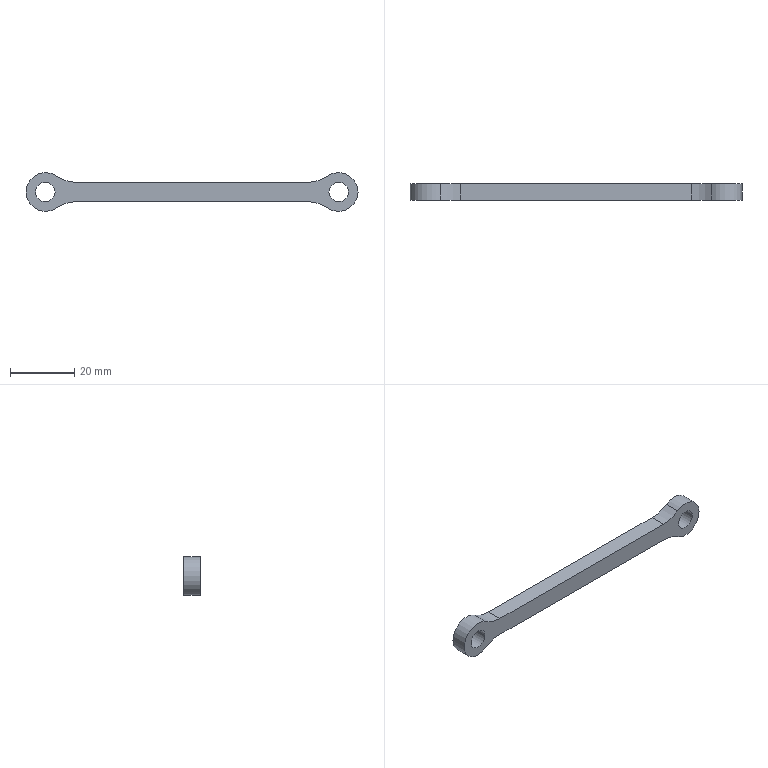Part | SolidWorks | features BaseBody 1 | 1 solid | 15 faces | box 103 x 5 x 12 mm | volume 3272 mm3 | cylinder 11 | plane 4 | commonest cylinder face diameters 6 x4 22 x4 12 x3
STEP:
#1=CARTESIAN_POINT('',(48.5,5.,0.));
#2=VERTEX_POINT('',#1);
#3=CARTESIAN_POINT('',(42.5,5.,0.));
#4=VERTEX_POINT('',#3);
#5=CARTESIAN_POINT('',(45.5,5.,0.));
#6=DIRECTION('',(0.,1.,0.));
#7=DIRECTION('',(1.,0.,0.));
#8=AXIS2_PLACEMENT_3D('',#5,#6,#7);
#9=CIRCLE('',#8,3.);
#10=EDGE_CURVE('',#2,#4,#9,.T.);
#11=ORIENTED_EDGE('',*,*,#10,.T.);
#12=CARTESIAN_POINT('',(42.5,0.,0.));
#13=VERTEX_POINT('',#12);
#14=CARTESIAN_POINT('',(42.5,5.,0.));
#15=DIRECTION('',(0.,-1.,0.));
#16=VECTOR('',#15,1000.);
#17=LINE('',#14,#16);
#18=EDGE_CURVE('',#4,#13,#17,.T.);
#19=ORIENTED_EDGE('',*,*,#18,.T.);
#20=CARTESIAN_POINT('',(48.5,0.,0.));
#21=VERTEX_POINT('',#20);
#22=CARTESIAN_POINT('',(45.5,0.,0.));
#23=DIRECTION('',(0.,-1.,0.));
#24=DIRECTION('',(1.,0.,0.));
#25=AXIS2_PLACEMENT_3D('',#22,#23,#24);
#26=CIRCLE('',#25,3.);
#27=EDGE_CURVE('',#13,#21,#26,.T.);
#28=ORIENTED_EDGE('',*,*,#27,.T.);
#29=CARTESIAN_POINT('',(48.5,5.,0.));
#30=DIRECTION('',(0.,-1.,0.));
#31=VECTOR('',#30,1000.);
#32=LINE('',#29,#31);
#33=EDGE_CURVE('',#2,#21,#32,.T.);
#34=ORIENTED_EDGE('',*,*,#33,.F.);
#35=EDGE_LOOP('',(#11,#19,#28,#34));
#36=FACE_OUTER_BOUND('',#35,.T.);
#37=CARTESIAN_POINT('',(45.5,5.,0.));
#38=DIRECTION('',(0.,-1.,0.));
#39=DIRECTION('',(1.,0.,0.));
#40=AXIS2_PLACEMENT_3D('',#37,#38,#39);
#41=CYLINDRICAL_SURFACE('',#40,3.);
#42=ADVANCED_FACE('',(#36),#41,.F.);
#43=CARTESIAN_POINT('',(-48.5,5.,0.));
#44=VERTEX_POINT('',#43);
#45=CARTESIAN_POINT('',(-42.5,5.,0.));
#46=VERTEX_POINT('',#45);
#47=CARTESIAN_POINT('',(-45.5,5.,0.));
#48=DIRECTION('',(0.,-1.,0.));
#49=DIRECTION('',(1.,0.,0.));
#50=AXIS2_PLACEMENT_3D('',#47,#48,#49);
#51=CIRCLE('',#50,3.);
#52=EDGE_CURVE('',#44,#46,#51,.T.);
#53=ORIENTED_EDGE('',*,*,#52,.F.);
#54=CARTESIAN_POINT('',(-48.5,0.,0.));
#55=VERTEX_POINT('',#54);
#56=CARTESIAN_POINT('',(-48.5,5.,0.));
#57=DIRECTION('',(0.,-1.,0.));
#58=VECTOR('',#57,1000.);
#59=LINE('',#56,#58);
#60=EDGE_CURVE('',#44,#55,#59,.T.);
#61=ORIENTED_EDGE('',*,*,#60,.T.);
#62=CARTESIAN_POINT('',(-42.5,0.,0.));
#63=VERTEX_POINT('',#62);
#64=CARTESIAN_POINT('',(-45.5,0.,0.));
#65=DIRECTION('',(0.,-1.,0.));
#66=DIRECTION('',(1.,0.,0.));
#67=AXIS2_PLACEMENT_3D('',#64,#65,#66);
#68=CIRCLE('',#67,3.);
#69=EDGE_CURVE('',#55,#63,#68,.T.);
#70=ORIENTED_EDGE('',*,*,#69,.T.);
#71=CARTESIAN_POINT('',(-42.5,5.,0.));
#72=DIRECTION('',(0.,-1.,0.));
#73=VECTOR('',#72,1000.);
#74=LINE('',#71,#73);
#75=EDGE_CURVE('',#46,#63,#74,.T.);
#76=ORIENTED_EDGE('',*,*,#75,.F.);
#77=EDGE_LOOP('',(#53,#61,#70,#76));
#78=FACE_OUTER_BOUND('',#77,.T.);
#79=CARTESIAN_POINT('',(-45.5,5.,0.));
#80=DIRECTION('',(0.,-1.,0.));
#81=DIRECTION('',(1.,0.,0.));
#82=AXIS2_PLACEMENT_3D('',#79,#80,#81);
#83=CYLINDRICAL_SURFACE('',#82,3.);
#84=ADVANCED_FACE('',(#78),#83,.F.);
#85=CARTESIAN_POINT('',(51.5,5.,0.));
#86=VERTEX_POINT('',#85);
#87=CARTESIAN_POINT('',(42.096,5.,-4.941));
#88=VERTEX_POINT('',#87);
#89=CARTESIAN_POINT('',(45.5,5.,0.));
#90=DIRECTION('',(0.,1.,0.));
#91=DIRECTION('',(1.,0.,0.));
#92=AXIS2_PLACEMENT_3D('',#89,#90,#91);
#93=CIRCLE('',#92,6.);
#94=EDGE_CURVE('',#86,#88,#93,.T.);
#95=ORIENTED_EDGE('',*,*,#94,.F.);
#96=CARTESIAN_POINT('',(51.5,0.,0.));
#97=VERTEX_POINT('',#96);
#98=CARTESIAN_POINT('',(51.5,5.,0.));
#99=DIRECTION('',(0.,-1.,0.));
#100=VECTOR('',#99,1000.);
#101=LINE('',#98,#100);
#102=EDGE_CURVE('',#86,#97,#101,.T.);
#103=ORIENTED_EDGE('',*,*,#102,.T.);
#104=CARTESIAN_POINT('',(42.096,0.,-4.941));
#105=VERTEX_POINT('',#104);
#106=CARTESIAN_POINT('',(45.5,0.,0.));
#107=DIRECTION('',(0.,1.,0.));
#108=DIRECTION('',(1.,0.,0.));
#109=AXIS2_PLACEMENT_3D('',#106,#107,#108);
#110=CIRCLE('',#109,6.);
#111=EDGE_CURVE('',#97,#105,#110,.T.);
#112=ORIENTED_EDGE('',*,*,#111,.T.);
#113=CARTESIAN_POINT('',(42.096,2.5,-4.941));
#114=DIRECTION('',(0.,-1.,0.));
#115=VECTOR('',#114,1000.);
#116=LINE('',#113,#115);
#117=EDGE_CURVE('',#88,#105,#116,.T.);
#118=ORIENTED_EDGE('',*,*,#117,.F.);
#119=EDGE_LOOP('',(#95,#103,#112,#118));
#120=FACE_OUTER_BOUND('',#119,.T.);
#121=CARTESIAN_POINT('',(45.5,5.,0.));
#122=DIRECTION('',(0.,-1.,0.));
#123=DIRECTION('',(1.,0.,0.));
#124=AXIS2_PLACEMENT_3D('',#121,#122,#123);
#125=CYLINDRICAL_SURFACE('',#124,6.);
#126=ADVANCED_FACE('',(#120),#125,.T.);
#127=ORIENTED_EDGE('',*,*,#18,.F.);
#128=CARTESIAN_POINT('',(45.5,5.,0.));
#129=DIRECTION('',(0.,1.,0.));
#130=DIRECTION('',(1.,0.,0.));
#131=AXIS2_PLACEMENT_3D('',#128,#129,#130);
#132=CIRCLE('',#131,3.);
#133=EDGE_CURVE('',#4,#2,#132,.T.);
#134=ORIENTED_EDGE('',*,*,#133,.T.);
#135=ORIENTED_EDGE('',*,*,#33,.T.);
#136=CARTESIAN_POINT('',(45.5,0.,0.));
#137=DIRECTION('',(0.,-1.,0.));
#138=DIRECTION('',(1.,0.,0.));
#139=AXIS2_PLACEMENT_3D('',#136,#137,#138);
#140=CIRCLE('',#139,3.);
#141=EDGE_CURVE('',#21,#13,#140,.T.);
#142=ORIENTED_EDGE('',*,*,#141,.T.);
#143=EDGE_LOOP('',(#127,#134,#135,#142));
#144=FACE_OUTER_BOUND('',#143,.T.);
#145=CARTESIAN_POINT('',(45.5,5.,0.));
#146=DIRECTION('',(0.,-1.,0.));
#147=DIRECTION('',(1.,0.,0.));
#148=AXIS2_PLACEMENT_3D('',#145,#146,#147);
#149=CYLINDRICAL_SURFACE('',#148,3.);
#150=ADVANCED_FACE('',(#144),#149,.F.);
#151=ORIENTED_EDGE('',*,*,#141,.F.);
#152=ORIENTED_EDGE('',*,*,#27,.F.);
#153=EDGE_LOOP('',(#151,#152));
#154=FACE_BOUND('',#153,.T.);
#155=CARTESIAN_POINT('',(-45.5,0.,0.));
#156=DIRECTION('',(0.,-1.,0.));
#157=DIRECTION('',(1.,0.,0.));
#158=AXIS2_PLACEMENT_3D('',#155,#156,#157);
#159=CIRCLE('',#158,3.);
#160=EDGE_CURVE('',#63,#55,#159,.T.);
#161=ORIENTED_EDGE('',*,*,#160,.F.);
#162=ORIENTED_EDGE('',*,*,#69,.F.);
#163=EDGE_LOOP('',(#161,#162));
#164=FACE_BOUND('',#163,.T.);
#165=CARTESIAN_POINT('',(42.096,0.,4.941));
#166=VERTEX_POINT('',#165);
#167=CARTESIAN_POINT('',(45.5,0.,0.));
#168=DIRECTION('',(0.,1.,0.));
#169=DIRECTION('',(1.,0.,0.));
#170=AXIS2_PLACEMENT_3D('',#167,#168,#169);
#171=CIRCLE('',#170,6.);
#172=EDGE_CURVE('',#166,#97,#171,.T.);
#173=ORIENTED_EDGE('',*,*,#172,.F.);
#174=CARTESIAN_POINT('',(35.856,0.,3.));
#175=VERTEX_POINT('',#174);
#176=CARTESIAN_POINT('',(35.856,0.,14.));
#177=DIRECTION('',(0.,-1.,0.));
#178=DIRECTION('',(1.,0.,0.));
#179=AXIS2_PLACEMENT_3D('',#176,#177,#178);
#180=CIRCLE('',#179,11.);
#181=EDGE_CURVE('',#175,#166,#180,.T.);
#182=ORIENTED_EDGE('',*,*,#181,.F.);
#183=CARTESIAN_POINT('',(-35.856,0.,3.));
#184=VERTEX_POINT('',#183);
#185=CARTESIAN_POINT('',(0.,0.,3.));
#186=DIRECTION('',(1.,0.,0.));
#187=VECTOR('',#186,1000.);
#188=LINE('',#185,#187);
#189=EDGE_CURVE('',#184,#175,#188,.T.);
#190=ORIENTED_EDGE('',*,*,#189,.F.);
#191=CARTESIAN_POINT('',(-42.096,0.,4.941));
#192=VERTEX_POINT('',#191);
#193=CARTESIAN_POINT('',(-35.856,0.,14.));
#194=DIRECTION('',(0.,-1.,0.));
#195=DIRECTION('',(1.,0.,0.));
#196=AXIS2_PLACEMENT_3D('',#193,#194,#195);
#197=CIRCLE('',#196,11.);
#198=EDGE_CURVE('',#192,#184,#197,.T.);
#199=ORIENTED_EDGE('',*,*,#198,.F.);
#200=CARTESIAN_POINT('',(-42.096,0.,-4.941));
#201=VERTEX_POINT('',#200);
#202=CARTESIAN_POINT('',(-45.5,0.,0.));
#203=DIRECTION('',(0.,1.,0.));
#204=DIRECTION('',(1.,0.,0.));
#205=AXIS2_PLACEMENT_3D('',#202,#203,#204);
#206=CIRCLE('',#205,6.);
#207=EDGE_CURVE('',#201,#192,#206,.T.);
#208=ORIENTED_EDGE('',*,*,#207,.F.);
#209=CARTESIAN_POINT('',(-35.856,0.,-3.));
#210=VERTEX_POINT('',#209);
#211=CARTESIAN_POINT('',(-35.856,0.,-14.));
#212=DIRECTION('',(0.,-1.,0.));
#213=DIRECTION('',(1.,0.,0.));
#214=AXIS2_PLACEMENT_3D('',#211,#212,#213);
#215=CIRCLE('',#214,11.);
#216=EDGE_CURVE('',#210,#201,#215,.T.);
#217=ORIENTED_EDGE('',*,*,#216,.F.);
#218=CARTESIAN_POINT('',(35.856,0.,-3.));
#219=VERTEX_POINT('',#218);
#220=CARTESIAN_POINT('',(0.,0.,-3.));
#221=DIRECTION('',(-1.,0.,0.));
#222=VECTOR('',#221,1000.);
#223=LINE('',#220,#222);
#224=EDGE_CURVE('',#219,#210,#223,.T.);
#225=ORIENTED_EDGE('',*,*,#224,.F.);
#226=CARTESIAN_POINT('',(35.856,0.,-14.));
#227=DIRECTION('',(0.,-1.,0.));
#228=DIRECTION('',(1.,0.,0.));
#229=AXIS2_PLACEMENT_3D('',#226,#227,#228);
#230=CIRCLE('',#229,11.);
#231=EDGE_CURVE('',#105,#219,#230,.T.);
#232=ORIENTED_EDGE('',*,*,#231,.F.);
#233=ORIENTED_EDGE('',*,*,#111,.F.);
#234=EDGE_LOOP('',(#173,#182,#190,#199,#208,#217,#225,#232,#233));
#235=FACE_OUTER_BOUND('',#234,.T.);
#236=CARTESIAN_POINT('',(-52.118,0.,-6.072));
#237=DIRECTION('',(0.,1.,0.));
#238=DIRECTION('',(0.,0.,1.));
#239=AXIS2_PLACEMENT_3D('',#236,#237,#238);
#240=PLANE('',#239);
#241=ADVANCED_FACE('',(#154,#164,#235),#240,.F.);
#242=ORIENTED_EDGE('',*,*,#10,.F.);
#243=ORIENTED_EDGE('',*,*,#133,.F.);
#244=EDGE_LOOP('',(#242,#243));
#245=FACE_BOUND('',#244,.T.);
#246=CARTESIAN_POINT('',(-45.5,5.,0.));
#247=DIRECTION('',(0.,-1.,0.));
#248=DIRECTION('',(1.,0.,0.));
#249=AXIS2_PLACEMENT_3D('',#246,#247,#248);
#250=CIRCLE('',#249,3.);
#251=EDGE_CURVE('',#46,#44,#250,.T.);
#252=ORIENTED_EDGE('',*,*,#251,.T.);
#253=ORIENTED_EDGE('',*,*,#52,.T.);
#254=EDGE_LOOP('',(#252,#253));
#255=FACE_BOUND('',#254,.T.);
#256=CARTESIAN_POINT('',(35.856,5.,3.));
#257=VERTEX_POINT('',#256);
#258=CARTESIAN_POINT('',(42.096,5.,4.941));
#259=VERTEX_POINT('',#258);
#260=CARTESIAN_POINT('',(35.856,5.,14.));
#261=DIRECTION('',(0.,-1.,0.));
#262=DIRECTION('',(1.,0.,0.));
#263=AXIS2_PLACEMENT_3D('',#260,#261,#262);
#264=CIRCLE('',#263,11.);
#265=EDGE_CURVE('',#257,#259,#264,.T.);
#266=ORIENTED_EDGE('',*,*,#265,.T.);
#267=CARTESIAN_POINT('',(45.5,5.,0.));
#268=DIRECTION('',(0.,1.,0.));
#269=DIRECTION('',(1.,0.,0.));
#270=AXIS2_PLACEMENT_3D('',#267,#268,#269);
#271=CIRCLE('',#270,6.);
#272=EDGE_CURVE('',#259,#86,#271,.T.);
#273=ORIENTED_EDGE('',*,*,#272,.T.);
#274=ORIENTED_EDGE('',*,*,#94,.T.);
#275=CARTESIAN_POINT('',(35.856,5.,-3.));
#276=VERTEX_POINT('',#275);
#277=CARTESIAN_POINT('',(35.856,5.,-14.));
#278=DIRECTION('',(0.,-1.,0.));
#279=DIRECTION('',(1.,0.,0.));
#280=AXIS2_PLACEMENT_3D('',#277,#278,#279);
#281=CIRCLE('',#280,11.);
#282=EDGE_CURVE('',#88,#276,#281,.T.);
#283=ORIENTED_EDGE('',*,*,#282,.T.);
#284=CARTESIAN_POINT('',(-35.856,5.,-3.));
#285=VERTEX_POINT('',#284);
#286=CARTESIAN_POINT('',(0.,5.,-3.));
#287=DIRECTION('',(-1.,0.,0.));
#288=VECTOR('',#287,1000.);
#289=LINE('',#286,#288);
#290=EDGE_CURVE('',#276,#285,#289,.T.);
#291=ORIENTED_EDGE('',*,*,#290,.T.);
#292=CARTESIAN_POINT('',(-42.096,5.,-4.941));
#293=VERTEX_POINT('',#292);
#294=CARTESIAN_POINT('',(-35.856,5.,-14.));
#295=DIRECTION('',(0.,-1.,0.));
#296=DIRECTION('',(1.,0.,0.));
#297=AXIS2_PLACEMENT_3D('',#294,#295,#296);
#298=CIRCLE('',#297,11.);
#299=EDGE_CURVE('',#285,#293,#298,.T.);
#300=ORIENTED_EDGE('',*,*,#299,.T.);
#301=CARTESIAN_POINT('',(-42.096,5.,4.941));
#302=VERTEX_POINT('',#301);
#303=CARTESIAN_POINT('',(-45.5,5.,0.));
#304=DIRECTION('',(0.,1.,0.));
#305=DIRECTION('',(1.,0.,0.));
#306=AXIS2_PLACEMENT_3D('',#303,#304,#305);
#307=CIRCLE('',#306,6.);
#308=EDGE_CURVE('',#293,#302,#307,.T.);
#309=ORIENTED_EDGE('',*,*,#308,.T.);
#310=CARTESIAN_POINT('',(-35.856,5.,3.));
#311=VERTEX_POINT('',#310);
#312=CARTESIAN_POINT('',(-35.856,5.,14.));
#313=DIRECTION('',(0.,-1.,0.));
#314=DIRECTION('',(1.,0.,0.));
#315=AXIS2_PLACEMENT_3D('',#312,#313,#314);
#316=CIRCLE('',#315,11.);
#317=EDGE_CURVE('',#302,#311,#316,.T.);
#318=ORIENTED_EDGE('',*,*,#317,.T.);
#319=CARTESIAN_POINT('',(0.,5.,3.));
#320=DIRECTION('',(1.,0.,0.));
#321=VECTOR('',#320,1000.);
#322=LINE('',#319,#321);
#323=EDGE_CURVE('',#311,#257,#322,.T.);
#324=ORIENTED_EDGE('',*,*,#323,.T.);
#325=EDGE_LOOP('',(#266,#273,#274,#283,#291,#300,#309,#318,#324));
#326=FACE_OUTER_BOUND('',#325,.T.);
#327=CARTESIAN_POINT('',(-52.118,5.,-6.072));
#328=DIRECTION('',(0.,1.,0.));
#329=DIRECTION('',(0.,0.,1.));
#330=AXIS2_PLACEMENT_3D('',#327,#328,#329);
#331=PLANE('',#330);
#332=ADVANCED_FACE('',(#245,#255,#326),#331,.T.);
#333=ORIENTED_EDGE('',*,*,#60,.F.);
#334=ORIENTED_EDGE('',*,*,#251,.F.);
#335=ORIENTED_EDGE('',*,*,#75,.T.);
#336=ORIENTED_EDGE('',*,*,#160,.T.);
#337=EDGE_LOOP('',(#333,#334,#335,#336));
#338=FACE_OUTER_BOUND('',#337,.T.);
#339=CARTESIAN_POINT('',(-45.5,5.,0.));
#340=DIRECTION('',(0.,-1.,0.));
#341=DIRECTION('',(1.,0.,0.));
#342=AXIS2_PLACEMENT_3D('',#339,#340,#341);
#343=CYLINDRICAL_SURFACE('',#342,3.);
#344=ADVANCED_FACE('',(#338),#343,.F.);
#345=ORIENTED_EDGE('',*,*,#282,.F.);
#346=ORIENTED_EDGE('',*,*,#117,.T.);
#347=ORIENTED_EDGE('',*,*,#231,.T.);
#348=CARTESIAN_POINT('',(35.856,2.5,-3.));
#349=DIRECTION('',(0.,1.,0.));
#350=VECTOR('',#349,1000.);
#351=LINE('',#348,#350);
#352=EDGE_CURVE('',#219,#276,#351,.T.);
#353=ORIENTED_EDGE('',*,*,#352,.T.);
#354=EDGE_LOOP('',(#345,#346,#347,#353));
#355=FACE_OUTER_BOUND('',#354,.T.);
#356=CARTESIAN_POINT('',(35.856,5.,-14.));
#357=DIRECTION('',(0.,-1.,0.));
#358=DIRECTION('',(1.,0.,0.));
#359=AXIS2_PLACEMENT_3D('',#356,#357,#358);
#360=CYLINDRICAL_SURFACE('',#359,11.);
#361=ADVANCED_FACE('',(#355),#360,.F.);
#362=ORIENTED_EDGE('',*,*,#102,.F.);
#363=ORIENTED_EDGE('',*,*,#272,.F.);
#364=CARTESIAN_POINT('',(42.096,2.5,4.941));
#365=DIRECTION('',(0.,1.,0.));
#366=VECTOR('',#365,1000.);
#367=LINE('',#364,#366);
#368=EDGE_CURVE('',#166,#259,#367,.T.);
#369=ORIENTED_EDGE('',*,*,#368,.F.);
#370=ORIENTED_EDGE('',*,*,#172,.T.);
#371=EDGE_LOOP('',(#362,#363,#369,#370));
#372=FACE_OUTER_BOUND('',#371,.T.);
#373=CARTESIAN_POINT('',(45.5,5.,0.));
#374=DIRECTION('',(0.,-1.,0.));
#375=DIRECTION('',(1.,0.,0.));
#376=AXIS2_PLACEMENT_3D('',#373,#374,#375);
#377=CYLINDRICAL_SURFACE('',#376,6.);
#378=ADVANCED_FACE('',(#372),#377,.T.);
#379=ORIENTED_EDGE('',*,*,#265,.F.);
#380=CARTESIAN_POINT('',(35.856,2.5,3.));
#381=DIRECTION('',(0.,-1.,0.));
#382=VECTOR('',#381,1000.);
#383=LINE('',#380,#382);
#384=EDGE_CURVE('',#257,#175,#383,.T.);
#385=ORIENTED_EDGE('',*,*,#384,.T.);
#386=ORIENTED_EDGE('',*,*,#181,.T.);
#387=ORIENTED_EDGE('',*,*,#368,.T.);
#388=EDGE_LOOP('',(#379,#385,#386,#387));
#389=FACE_OUTER_BOUND('',#388,.T.);
#390=CARTESIAN_POINT('',(35.856,5.,14.));
#391=DIRECTION('',(0.,-1.,0.));
#392=DIRECTION('',(1.,0.,0.));
#393=AXIS2_PLACEMENT_3D('',#390,#391,#392);
#394=CYLINDRICAL_SURFACE('',#393,11.);
#395=ADVANCED_FACE('',(#389),#394,.F.);
#396=ORIENTED_EDGE('',*,*,#384,.F.);
#397=ORIENTED_EDGE('',*,*,#323,.F.);
#398=CARTESIAN_POINT('',(-35.856,2.5,3.));
#399=DIRECTION('',(0.,1.,0.));
#400=VECTOR('',#399,1000.);
#401=LINE('',#398,#400);
#402=EDGE_CURVE('',#184,#311,#401,.T.);
#403=ORIENTED_EDGE('',*,*,#402,.F.);
#404=ORIENTED_EDGE('',*,*,#189,.T.);
#405=EDGE_LOOP('',(#396,#397,#403,#404));
#406=FACE_OUTER_BOUND('',#405,.T.);
#407=CARTESIAN_POINT('',(35.856,0.,3.));
#408=DIRECTION('',(0.,0.,-1.));
#409=DIRECTION('',(-1.,0.,0.));
#410=AXIS2_PLACEMENT_3D('',#407,#408,#409);
#411=PLANE('',#410);
#412=ADVANCED_FACE('',(#406),#411,.F.);
#413=ORIENTED_EDGE('',*,*,#317,.F.);
#414=CARTESIAN_POINT('',(-42.096,2.5,4.941));
#415=DIRECTION('',(0.,-1.,0.));
#416=VECTOR('',#415,1000.);
#417=LINE('',#414,#416);
#418=EDGE_CURVE('',#302,#192,#417,.T.);
#419=ORIENTED_EDGE('',*,*,#418,.T.);
#420=ORIENTED_EDGE('',*,*,#198,.T.);
#421=ORIENTED_EDGE('',*,*,#402,.T.);
#422=EDGE_LOOP('',(#413,#419,#420,#421));
#423=FACE_OUTER_BOUND('',#422,.T.);
#424=CARTESIAN_POINT('',(-35.856,5.,14.));
#425=DIRECTION('',(0.,-1.,0.));
#426=DIRECTION('',(1.,0.,0.));
#427=AXIS2_PLACEMENT_3D('',#424,#425,#426);
#428=CYLINDRICAL_SURFACE('',#427,11.);
#429=ADVANCED_FACE('',(#423),#428,.F.);
#430=ORIENTED_EDGE('',*,*,#308,.F.);
#431=CARTESIAN_POINT('',(-42.096,2.5,-4.941));
#432=DIRECTION('',(0.,1.,0.));
#433=VECTOR('',#432,1000.);
#434=LINE('',#431,#433);
#435=EDGE_CURVE('',#201,#293,#434,.T.);
#436=ORIENTED_EDGE('',*,*,#435,.F.);
#437=ORIENTED_EDGE('',*,*,#207,.T.);
#438=ORIENTED_EDGE('',*,*,#418,.F.);
#439=EDGE_LOOP('',(#430,#436,#437,#438));
#440=FACE_OUTER_BOUND('',#439,.T.);
#441=CARTESIAN_POINT('',(-45.5,5.,0.));
#442=DIRECTION('',(0.,-1.,0.));
#443=DIRECTION('',(1.,0.,0.));
#444=AXIS2_PLACEMENT_3D('',#441,#442,#443);
#445=CYLINDRICAL_SURFACE('',#444,6.);
#446=ADVANCED_FACE('',(#440),#445,.T.);
#447=ORIENTED_EDGE('',*,*,#299,.F.);
#448=CARTESIAN_POINT('',(-35.856,2.5,-3.));
#449=DIRECTION('',(0.,-1.,0.));
#450=VECTOR('',#449,1000.);
#451=LINE('',#448,#450);
#452=EDGE_CURVE('',#285,#210,#451,.T.);
#453=ORIENTED_EDGE('',*,*,#452,.T.);
#454=ORIENTED_EDGE('',*,*,#216,.T.);
#455=ORIENTED_EDGE('',*,*,#435,.T.);
#456=EDGE_LOOP('',(#447,#453,#454,#455));
#457=FACE_OUTER_BOUND('',#456,.T.);
#458=CARTESIAN_POINT('',(-35.856,5.,-14.));
#459=DIRECTION('',(0.,-1.,0.));
#460=DIRECTION('',(1.,0.,0.));
#461=AXIS2_PLACEMENT_3D('',#458,#459,#460);
#462=CYLINDRICAL_SURFACE('',#461,11.);
#463=ADVANCED_FACE('',(#457),#462,.F.);
#464=ORIENTED_EDGE('',*,*,#452,.F.);
#465=ORIENTED_EDGE('',*,*,#290,.F.);
#466=ORIENTED_EDGE('',*,*,#352,.F.);
#467=ORIENTED_EDGE('',*,*,#224,.T.);
#468=EDGE_LOOP('',(#464,#465,#466,#467));
#469=FACE_OUTER_BOUND('',#468,.T.);
#470=CARTESIAN_POINT('',(-35.856,0.,-3.));
#471=DIRECTION('',(0.,0.,1.));
#472=DIRECTION('',(1.,0.,0.));
#473=AXIS2_PLACEMENT_3D('',#470,#471,#472);
#474=PLANE('',#473);
#475=ADVANCED_FACE('',(#469),#474,.F.);
#476=CLOSED_SHELL('',(#42,#84,#126,#150,#241,#332,#344,#361,#378,#395,#412,#429,#446,#463,#475));
#477=MANIFOLD_SOLID_BREP('',#476);
#478=CARTESIAN_POINT('',(0.,0.,0.));
#479=DIRECTION('',(0.,0.,1.));
#480=DIRECTION('',(1.,0.,0.));
#481=AXIS2_PLACEMENT_3D('',#478,#479,#480);
#482=(LENGTH_UNIT()NAMED_UNIT(*)SI_UNIT(.MILLI.,.METRE.));
#483=UNCERTAINTY_MEASURE_WITH_UNIT(LENGTH_MEASURE(0.00001),#482,'','');
#484=(NAMED_UNIT(*)PLANE_ANGLE_UNIT()SI_UNIT($,.RADIAN.));
#485=(NAMED_UNIT(*)SI_UNIT($,.STERADIAN.)SOLID_ANGLE_UNIT());
#486=(GEOMETRIC_REPRESENTATION_CONTEXT(3)GLOBAL_UNCERTAINTY_ASSIGNED_CONTEXT((#483))GLOBAL_UNIT_ASSIGNED_CONTEXT((#482,#484,#485))REPRESENTATION_CONTEXT('',''));
#487=ADVANCED_BREP_SHAPE_REPRESENTATION('',(#477,#481),#486);